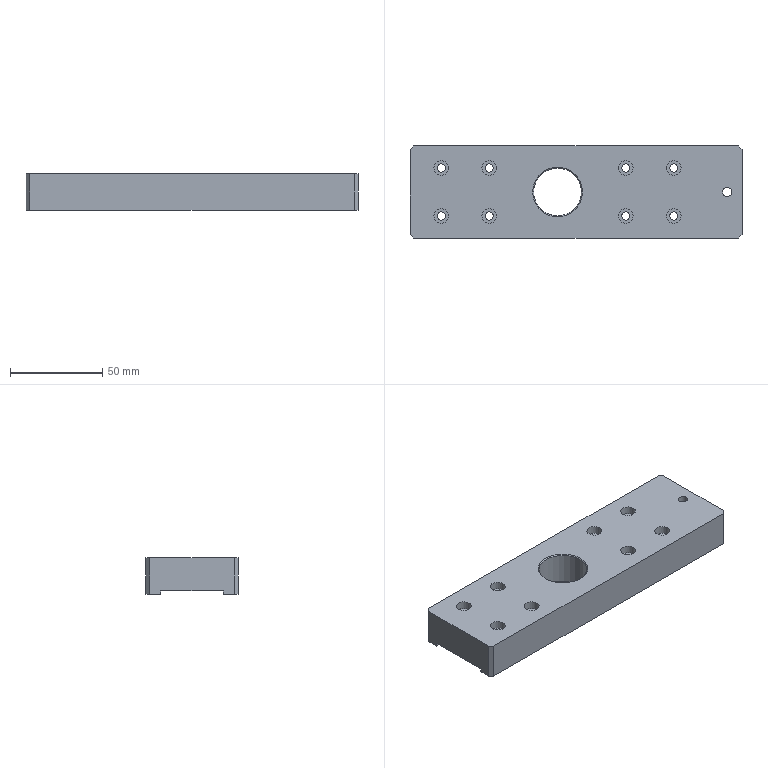CAM job | NX | 3-axis milling, drilling | part box 180 x 50 x 20 mm | stock box 180 x 50 x 20 mm
Tools:
number,name,description,diameter,corner_radius,flute_length,length,flutes
4,D4,平底铣刀-粗,4.0,0.0,25.0,75.0,2
9,D10,平底铣刀-粗,10.0,0.0,35.0,75.0,2
11,D4-J,平底铣刀-精,4.0,0.0,50.0,75.0,2
10,D10-J,平底铣刀-精,10.0,0.0,35.0,75.0,2
2,D6倒角刀,倒角刀,6.0,0.0,3.0,25.0,2
23,M6X1.0,丝锥,5.0,0.0,35.0,50.0,2
1,C6定点钻,倒角刀,6.0,0.0,3.0,3.0,2
11,ZT4.5,钻头,4.5,0.0,35.0,50.0,2
15,ZT5.1,钻头,5.1,0.0,35.0,50.0,2
19,ZT10,钻头,10.0,0.0,35.0,50.0,2
Operations:
program,operation,operation_type,tool,method,geometry_group,spindle_rpm,surface_speed,feed_per_tooth,feed_cut,feed_plunge,cut_length_mm,path_length_mm,cut_time_min,machine_time_min
B,选线往复层切开粗-中_COPY_1,PlanarMilling,D10,分层开粗-切深K-步距G,W-B,3000.0,94.245,0.3333,2000.0,100.0,1832.902,2460.185,0.9165,0.9792
B,底壁铣分层开粗-中_COPY,VolumeBased25DMillingOperation,D10,分层开粗-切深K-步距G,W-B,3000.0,94.245,0.3333,2000.0,100.0,7316.298,7339.806,3.658,3.66
B,钻倒角_1,Operation,D6倒角刀,METHOD,W-B,2000.0,0.0,0.025,100.0,0.0,44.4,404.696,0.444,0.48
B,铣倒角_2,PlanarMilling,D6倒角刀,METHOD,W-B,4000.0,75.398,0.0375,300.0,100.0,18.02,84.02,0.0601,0.0667
B,底壁铣倒角_COPY,VolumeBased25DMillingOperation,D6倒角刀,爬面_倒角-切深0-步距G,W-B,3500.0,65.972,0.1429,1000.0,100.0,84.583,147.983,0.0846,0.0909
B,平面去毛刺6X45L_COPY_1,SurfaceContour,D6倒角刀,爬面_倒角-切深0-步距G,W-B,3500.0,65.972,0.1429,1000.0,100.0,917.177,1837.503,0.9172,1.009
B,底壁铣精光底面-中_COPY,VolumeBased25DMillingOperation,D10-J,精光步距切深关,W-B,3000.0,94.245,0.1333,800.0,100.0,1128.98,1150.58,1.411,1.413
B,底壁铣精光侧面-中-选底面_COPY,VolumeBased25DMillingOperation,D10-J,侧刃精光-切深K-步距G,W-B,3000.0,94.245,0.1333,800.0,100.0,397.362,438.764,0.4967,0.5008
B,平面铣精光侧面-中-直线_COPY_1,PlanarMilling,D10-J,侧刃精光-切深K-步距G,W-B,3000.0,94.245,0.1333,800.0,100.0,67.314,651.071,0.0841,0.1425
A,打点-深0.8,Operation,C6定点钻,NONE,W-A,3000.0,56.0,0.01,60.0,90.0,18.0,371.372,0.3,0.3353
A,通孔-M6螺纹底孔,Operation,ZT5.1,NONE,W-A,800.0,12.566,0.0625,100.0,90.0,26.0,112.0,0.26,0.2686
A,沉头孔-钻孔0段,Operation,ZT4.5,NONE,W-A,800.0,11.31,0.0375,60.0,90.0,179.615,656.353,2.994,3.041
A,铣孔开粗D4_1,CylinderMilling,D4,NONE,W-A,4000.0,50.266,0.1875,1500.0,100.0,2483.443,3224.643,1.656,1.73
A,铣孔精光D4_1,CylinderMilling,D4-J,精光步距切深关,W-A,4000.0,50.266,0.1,800.0,100.0,256.369,997.569,0.3205,0.3946
A,通孔-精孔12.0预钻,Operation,ZT10,NONE,W-A,500.0,40.526,0.12,120.0,90.0,26.0,112.0,0.2167,0.2253
A,选线往复层切开粗-中_COPY,PlanarMilling,D10,分层开粗-切深K-步距G,W-A,3000.0,94.245,0.3333,2000.0,100.0,1832.902,2460.185,0.9165,0.9792
A,底壁铣螺旋开粗-中_COPY,VolumeBased25DMillingOperation,D10,分层开粗-切深K-步距G,W-A,3000.0,94.245,0.3333,2000.0,100.0,4865.824,4942.924,2.433,2.441
A,铣倒角_1,PlanarMilling,D6倒角刀,METHOD,W-A,4000.0,75.398,0.0375,300.0,100.0,19.938,81.138,0.0665,0.0726
A,铣倒角_3,PlanarMilling,D6倒角刀,METHOD,W-A,4000.0,75.398,0.1,800.0,100.0,85.823,147.823,0.1073,0.1135
A,平面去毛刺6X45L_COPY,SurfaceContour,D6倒角刀,爬面_倒角-切深0-步距G,W-A,3500.0,65.972,0.1429,1000.0,100.0,659.622,1246.891,0.6596,0.7183
A,通孔-攻牙M6,Operation,M6X1.0,METHOD,W-A,400.0,6.283,0.0013,1.0,90.0,23.0,106.0,23.0,23.008
A,底壁铣精光侧面-中_COPY,VolumeBased25DMillingOperation,D10-J,侧刃精光-切深K-步距G,W-A,3000.0,94.245,0.1333,800.0,100.0,177.667,233.519,0.2221,0.2277
A,平面铣精光侧面-中-直线_COPY,PlanarMilling,D10-J,侧刃精光-切深K-步距G,W-A,3000.0,94.245,0.1333,800.0,100.0,67.314,651.071,0.0841,0.1425